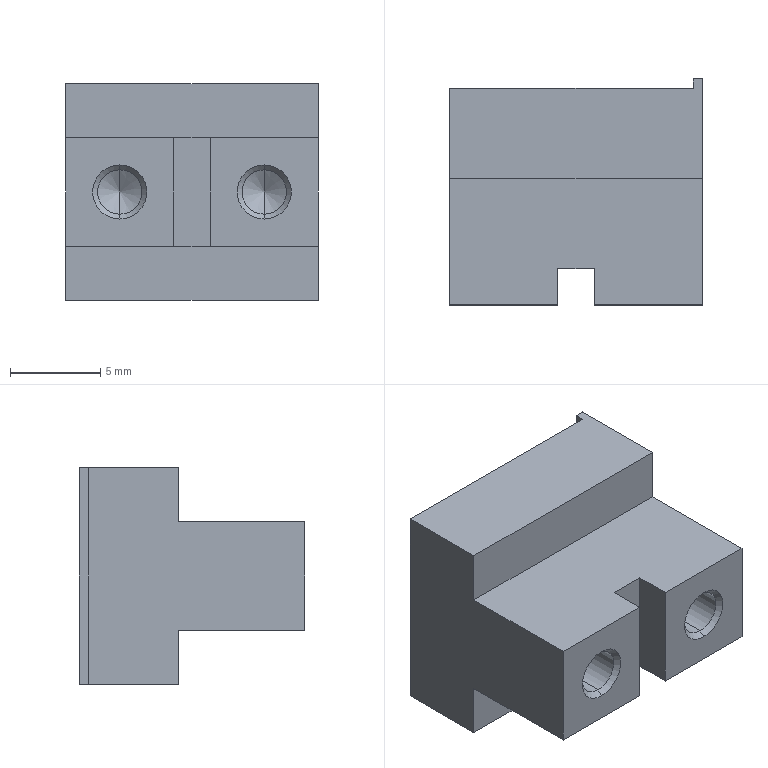Part | SolidWorks | features BaseBody 1 | 1 solid | 28 faces | box 14 x 12.5 x 12 mm | volume 1347 mm3 | plane 16 | cone 8 | cylinder 4 | commonest cylinder face diameters 2.459 x4
STEP:
#1=CARTESIAN_POINT('',(-11.,-11.729,1.229));
#2=VERTEX_POINT('',#1);
#3=CARTESIAN_POINT('',(-11.,-11.729,-1.229));
#4=VERTEX_POINT('',#3);
#5=CARTESIAN_POINT('',(-11.,-11.729,0.));
#6=DIRECTION('',(0.,-1.,0.));
#7=DIRECTION('',(0.,0.,-1.));
#8=AXIS2_PLACEMENT_3D('',#5,#6,#7);
#9=CIRCLE('',#8,1.229);
#10=EDGE_CURVE('',#2,#4,#9,.T.);
#11=ORIENTED_EDGE('',*,*,#10,.F.);
#12=CARTESIAN_POINT('',(-11.,-12.,1.5));
#13=VERTEX_POINT('',#12);
#14=CARTESIAN_POINT('',(-11.,-11.729,1.229));
#15=DIRECTION('',(0.,-0.7071,0.7071));
#16=VECTOR('',#15,1000.);
#17=LINE('',#14,#16);
#18=EDGE_CURVE('',#2,#13,#17,.T.);
#19=ORIENTED_EDGE('',*,*,#18,.T.);
#20=CARTESIAN_POINT('',(-11.,-12.,-1.5));
#21=VERTEX_POINT('',#20);
#22=CARTESIAN_POINT('',(-11.,-12.,0.));
#23=DIRECTION('',(0.,-1.,0.));
#24=DIRECTION('',(0.,0.,-1.));
#25=AXIS2_PLACEMENT_3D('',#22,#23,#24);
#26=CIRCLE('',#25,1.5);
#27=EDGE_CURVE('',#13,#21,#26,.T.);
#28=ORIENTED_EDGE('',*,*,#27,.T.);
#29=CARTESIAN_POINT('',(-11.,-11.729,-1.229));
#30=DIRECTION('',(0.,-0.7071,-0.7071));
#31=VECTOR('',#30,1000.);
#32=LINE('',#29,#31);
#33=EDGE_CURVE('',#4,#21,#32,.T.);
#34=ORIENTED_EDGE('',*,*,#33,.F.);
#35=EDGE_LOOP('',(#11,#19,#28,#34));
#36=FACE_OUTER_BOUND('',#35,.T.);
#37=CARTESIAN_POINT('',(-11.,-11.729,0.));
#38=DIRECTION('',(0.,-1.,0.));
#39=DIRECTION('',(0.,0.,-1.));
#40=AXIS2_PLACEMENT_3D('',#37,#38,#39);
#41=CONICAL_SURFACE('',#40,1.229,0.7854);
#42=ADVANCED_FACE('',(#36),#41,.F.);
#43=CARTESIAN_POINT('',(-11.,-6.,1.229));
#44=VERTEX_POINT('',#43);
#45=CARTESIAN_POINT('',(-11.,-6.,-1.229));
#46=VERTEX_POINT('',#45);
#47=CARTESIAN_POINT('',(-11.,-6.,0.));
#48=DIRECTION('',(0.,-1.,0.));
#49=DIRECTION('',(0.,0.,-1.));
#50=AXIS2_PLACEMENT_3D('',#47,#48,#49);
#51=CIRCLE('',#50,1.229);
#52=EDGE_CURVE('',#44,#46,#51,.T.);
#53=ORIENTED_EDGE('',*,*,#52,.F.);
#54=CARTESIAN_POINT('',(-11.,-12.,1.229));
#55=DIRECTION('',(0.,-1.,0.));
#56=VECTOR('',#55,1000.);
#57=LINE('',#54,#56);
#58=EDGE_CURVE('',#44,#2,#57,.T.);
#59=ORIENTED_EDGE('',*,*,#58,.T.);
#60=ORIENTED_EDGE('',*,*,#10,.T.);
#61=CARTESIAN_POINT('',(-11.,-12.,-1.229));
#62=DIRECTION('',(0.,-1.,0.));
#63=VECTOR('',#62,1000.);
#64=LINE('',#61,#63);
#65=EDGE_CURVE('',#46,#4,#64,.T.);
#66=ORIENTED_EDGE('',*,*,#65,.F.);
#67=EDGE_LOOP('',(#53,#59,#60,#66));
#68=FACE_OUTER_BOUND('',#67,.T.);
#69=CARTESIAN_POINT('',(-11.,-12.,0.));
#70=DIRECTION('',(0.,-1.,0.));
#71=DIRECTION('',(0.,0.,-1.));
#72=AXIS2_PLACEMENT_3D('',#69,#70,#71);
#73=CYLINDRICAL_SURFACE('',#72,1.229);
#74=ADVANCED_FACE('',(#68),#73,.F.);
#75=CARTESIAN_POINT('',(-11.,-5.29,0.));
#76=VERTEX_POINT('',#75);
#77=CARTESIAN_POINT('',(-11.,-5.29,0.));
#78=DIRECTION('',(0.,-0.5,-0.866));
#79=VECTOR('',#78,1000.);
#80=LINE('',#77,#79);
#81=EDGE_CURVE('',#76,#46,#80,.T.);
#82=ORIENTED_EDGE('',*,*,#81,.F.);
#83=CARTESIAN_POINT('',(-11.,-5.29,0.));
#84=DIRECTION('',(0.,-0.5,0.866));
#85=VECTOR('',#84,1000.);
#86=LINE('',#83,#85);
#87=EDGE_CURVE('',#76,#44,#86,.T.);
#88=ORIENTED_EDGE('',*,*,#87,.T.);
#89=ORIENTED_EDGE('',*,*,#52,.T.);
#90=EDGE_LOOP('',(#82,#88,#89));
#91=FACE_OUTER_BOUND('',#90,.T.);
#92=CARTESIAN_POINT('',(-11.,-1005.29,0.));
#93=DIRECTION('',(0.,-1.,0.));
#94=DIRECTION('',(0.,0.,-1.));
#95=AXIS2_PLACEMENT_3D('',#92,#93,#94);
#96=CONICAL_SURFACE('',#95,1732.051,1.047);
#97=ADVANCED_FACE('',(#91),#96,.F.);
#98=CARTESIAN_POINT('',(-3.,-11.729,1.229));
#99=VERTEX_POINT('',#98);
#100=CARTESIAN_POINT('',(-3.,-11.729,-1.229));
#101=VERTEX_POINT('',#100);
#102=CARTESIAN_POINT('',(-3.,-11.729,0.));
#103=DIRECTION('',(0.,-1.,0.));
#104=DIRECTION('',(0.,0.,-1.));
#105=AXIS2_PLACEMENT_3D('',#102,#103,#104);
#106=CIRCLE('',#105,1.229);
#107=EDGE_CURVE('',#99,#101,#106,.T.);
#108=ORIENTED_EDGE('',*,*,#107,.F.);
#109=CARTESIAN_POINT('',(-3.,-12.,1.5));
#110=VERTEX_POINT('',#109);
#111=CARTESIAN_POINT('',(-3.,-11.729,1.229));
#112=DIRECTION('',(0.,-0.7071,0.7071));
#113=VECTOR('',#112,1000.);
#114=LINE('',#111,#113);
#115=EDGE_CURVE('',#99,#110,#114,.T.);
#116=ORIENTED_EDGE('',*,*,#115,.T.);
#117=CARTESIAN_POINT('',(-3.,-12.,-1.5));
#118=VERTEX_POINT('',#117);
#119=CARTESIAN_POINT('',(-3.,-12.,0.));
#120=DIRECTION('',(0.,-1.,0.));
#121=DIRECTION('',(0.,0.,-1.));
#122=AXIS2_PLACEMENT_3D('',#119,#120,#121);
#123=CIRCLE('',#122,1.5);
#124=EDGE_CURVE('',#110,#118,#123,.T.);
#125=ORIENTED_EDGE('',*,*,#124,.T.);
#126=CARTESIAN_POINT('',(-3.,-11.729,-1.229));
#127=DIRECTION('',(0.,-0.7071,-0.7071));
#128=VECTOR('',#127,1000.);
#129=LINE('',#126,#128);
#130=EDGE_CURVE('',#101,#118,#129,.T.);
#131=ORIENTED_EDGE('',*,*,#130,.F.);
#132=EDGE_LOOP('',(#108,#116,#125,#131));
#133=FACE_OUTER_BOUND('',#132,.T.);
#134=CARTESIAN_POINT('',(-3.,-11.729,0.));
#135=DIRECTION('',(0.,-1.,0.));
#136=DIRECTION('',(0.,0.,-1.));
#137=AXIS2_PLACEMENT_3D('',#134,#135,#136);
#138=CONICAL_SURFACE('',#137,1.229,0.7854);
#139=ADVANCED_FACE('',(#133),#138,.F.);
#140=CARTESIAN_POINT('',(-3.,-6.,1.229));
#141=VERTEX_POINT('',#140);
#142=CARTESIAN_POINT('',(-3.,-6.,-1.229));
#143=VERTEX_POINT('',#142);
#144=CARTESIAN_POINT('',(-3.,-6.,0.));
#145=DIRECTION('',(0.,-1.,0.));
#146=DIRECTION('',(0.,0.,-1.));
#147=AXIS2_PLACEMENT_3D('',#144,#145,#146);
#148=CIRCLE('',#147,1.229);
#149=EDGE_CURVE('',#141,#143,#148,.T.);
#150=ORIENTED_EDGE('',*,*,#149,.F.);
#151=CARTESIAN_POINT('',(-3.,-12.,1.229));
#152=DIRECTION('',(0.,-1.,0.));
#153=VECTOR('',#152,1000.);
#154=LINE('',#151,#153);
#155=EDGE_CURVE('',#141,#99,#154,.T.);
#156=ORIENTED_EDGE('',*,*,#155,.T.);
#157=ORIENTED_EDGE('',*,*,#107,.T.);
#158=CARTESIAN_POINT('',(-3.,-12.,-1.229));
#159=DIRECTION('',(0.,-1.,0.));
#160=VECTOR('',#159,1000.);
#161=LINE('',#158,#160);
#162=EDGE_CURVE('',#143,#101,#161,.T.);
#163=ORIENTED_EDGE('',*,*,#162,.F.);
#164=EDGE_LOOP('',(#150,#156,#157,#163));
#165=FACE_OUTER_BOUND('',#164,.T.);
#166=CARTESIAN_POINT('',(-3.,-12.,0.));
#167=DIRECTION('',(0.,-1.,0.));
#168=DIRECTION('',(0.,0.,-1.));
#169=AXIS2_PLACEMENT_3D('',#166,#167,#168);
#170=CYLINDRICAL_SURFACE('',#169,1.229);
#171=ADVANCED_FACE('',(#165),#170,.F.);
#172=CARTESIAN_POINT('',(-3.,-5.29,0.));
#173=VERTEX_POINT('',#172);
#174=CARTESIAN_POINT('',(-3.,-5.29,0.));
#175=DIRECTION('',(0.,-0.5,-0.866));
#176=VECTOR('',#175,1000.);
#177=LINE('',#174,#176);
#178=EDGE_CURVE('',#173,#143,#177,.T.);
#179=ORIENTED_EDGE('',*,*,#178,.F.);
#180=CARTESIAN_POINT('',(-3.,-5.29,0.));
#181=DIRECTION('',(0.,-0.5,0.866));
#182=VECTOR('',#181,1000.);
#183=LINE('',#180,#182);
#184=EDGE_CURVE('',#173,#141,#183,.T.);
#185=ORIENTED_EDGE('',*,*,#184,.T.);
#186=ORIENTED_EDGE('',*,*,#149,.T.);
#187=EDGE_LOOP('',(#179,#185,#186));
#188=FACE_OUTER_BOUND('',#187,.T.);
#189=CARTESIAN_POINT('',(-3.,-1005.29,0.));
#190=DIRECTION('',(0.,-1.,0.));
#191=DIRECTION('',(0.,0.,-1.));
#192=AXIS2_PLACEMENT_3D('',#189,#190,#191);
#193=CONICAL_SURFACE('',#192,1732.051,1.047);
#194=ADVANCED_FACE('',(#188),#193,.F.);
#195=CARTESIAN_POINT('',(-3.,-12.,0.));
#196=DIRECTION('',(0.,-1.,0.));
#197=DIRECTION('',(0.,0.,-1.));
#198=AXIS2_PLACEMENT_3D('',#195,#196,#197);
#199=CIRCLE('',#198,1.5);
#200=EDGE_CURVE('',#118,#110,#199,.T.);
#201=ORIENTED_EDGE('',*,*,#200,.F.);
#202=ORIENTED_EDGE('',*,*,#124,.F.);
#203=EDGE_LOOP('',(#201,#202));
#204=FACE_BOUND('',#203,.T.);
#205=CARTESIAN_POINT('',(-6.,-12.,-3.));
#206=VERTEX_POINT('',#205);
#207=CARTESIAN_POINT('',(-6.,-12.,3.));
#208=VERTEX_POINT('',#207);
#209=CARTESIAN_POINT('',(-6.,-12.,-3.));
#210=DIRECTION('',(0.,0.,1.));
#211=VECTOR('',#210,1000.);
#212=LINE('',#209,#211);
#213=EDGE_CURVE('',#206,#208,#212,.T.);
#214=ORIENTED_EDGE('',*,*,#213,.F.);
#215=CARTESIAN_POINT('',(0.,-12.,-3.));
#216=VERTEX_POINT('',#215);
#217=CARTESIAN_POINT('',(-6.,-12.,-3.));
#218=DIRECTION('',(1.,0.,0.));
#219=VECTOR('',#218,1000.);
#220=LINE('',#217,#219);
#221=EDGE_CURVE('',#206,#216,#220,.T.);
#222=ORIENTED_EDGE('',*,*,#221,.T.);
#223=CARTESIAN_POINT('',(0.,-12.,3.));
#224=VERTEX_POINT('',#223);
#225=CARTESIAN_POINT('',(0.,-12.,3.));
#226=DIRECTION('',(0.,0.,-1.));
#227=VECTOR('',#226,1000.);
#228=LINE('',#225,#227);
#229=EDGE_CURVE('',#224,#216,#228,.T.);
#230=ORIENTED_EDGE('',*,*,#229,.F.);
#231=CARTESIAN_POINT('',(-6.,-12.,3.));
#232=DIRECTION('',(1.,0.,0.));
#233=VECTOR('',#232,1000.);
#234=LINE('',#231,#233);
#235=EDGE_CURVE('',#208,#224,#234,.T.);
#236=ORIENTED_EDGE('',*,*,#235,.F.);
#237=EDGE_LOOP('',(#214,#222,#230,#236));
#238=FACE_OUTER_BOUND('',#237,.T.);
#239=CARTESIAN_POINT('',(-14.,-12.,3.));
#240=DIRECTION('',(0.,-1.,0.));
#241=DIRECTION('',(0.,0.,-1.));
#242=AXIS2_PLACEMENT_3D('',#239,#240,#241);
#243=PLANE('',#242);
#244=ADVANCED_FACE('',(#204,#238),#243,.T.);
#245=CARTESIAN_POINT('',(-14.,0.,6.));
#246=VERTEX_POINT('',#245);
#247=CARTESIAN_POINT('',(-0.5,0.,6.));
#248=VERTEX_POINT('',#247);
#249=CARTESIAN_POINT('',(-14.,0.,6.));
#250=DIRECTION('',(1.,0.,0.));
#251=VECTOR('',#250,1000.);
#252=LINE('',#249,#251);
#253=EDGE_CURVE('',#246,#248,#252,.T.);
#254=ORIENTED_EDGE('',*,*,#253,.T.);
#255=CARTESIAN_POINT('',(-0.5,0.,-6.));
#256=VERTEX_POINT('',#255);
#257=CARTESIAN_POINT('',(-0.5,0.,6.));
#258=DIRECTION('',(0.,0.,-1.));
#259=VECTOR('',#258,1000.);
#260=LINE('',#257,#259);
#261=EDGE_CURVE('',#248,#256,#260,.T.);
#262=ORIENTED_EDGE('',*,*,#261,.T.);
#263=CARTESIAN_POINT('',(-14.,0.,-6.));
#264=VERTEX_POINT('',#263);
#265=CARTESIAN_POINT('',(-14.,0.,-6.));
#266=DIRECTION('',(1.,0.,0.));
#267=VECTOR('',#266,1000.);
#268=LINE('',#265,#267);
#269=EDGE_CURVE('',#264,#256,#268,.T.);
#270=ORIENTED_EDGE('',*,*,#269,.F.);
#271=CARTESIAN_POINT('',(-14.,0.,-6.));
#272=DIRECTION('',(0.,0.,1.));
#273=VECTOR('',#272,1000.);
#274=LINE('',#271,#273);
#275=EDGE_CURVE('',#264,#246,#274,.T.);
#276=ORIENTED_EDGE('',*,*,#275,.T.);
#277=EDGE_LOOP('',(#254,#262,#270,#276));
#278=FACE_OUTER_BOUND('',#277,.T.);
#279=CARTESIAN_POINT('',(-14.,0.,-6.));
#280=DIRECTION('',(0.,1.,0.));
#281=DIRECTION('',(0.,0.,1.));
#282=AXIS2_PLACEMENT_3D('',#279,#280,#281);
#283=PLANE('',#282);
#284=ADVANCED_FACE('',(#278),#283,.T.);
#285=CARTESIAN_POINT('',(0.,0.5,6.));
#286=VERTEX_POINT('',#285);
#287=CARTESIAN_POINT('',(0.,-5.,6.));
#288=VERTEX_POINT('',#287);
#289=CARTESIAN_POINT('',(0.,0.5,6.));
#290=DIRECTION('',(0.,-1.,0.));
#291=VECTOR('',#290,1000.);
#292=LINE('',#289,#291);
#293=EDGE_CURVE('',#286,#288,#292,.T.);
#294=ORIENTED_EDGE('',*,*,#293,.F.);
#295=CARTESIAN_POINT('',(-0.5,0.5,6.));
#296=VERTEX_POINT('',#295);
#297=CARTESIAN_POINT('',(-0.5,0.5,6.));
#298=DIRECTION('',(1.,0.,0.));
#299=VECTOR('',#298,1000.);
#300=LINE('',#297,#299);
#301=EDGE_CURVE('',#296,#286,#300,.T.);
#302=ORIENTED_EDGE('',*,*,#301,.F.);
#303=CARTESIAN_POINT('',(-0.5,0.5,6.));
#304=DIRECTION('',(0.,-1.,0.));
#305=VECTOR('',#304,1000.);
#306=LINE('',#303,#305);
#307=EDGE_CURVE('',#296,#248,#306,.T.);
#308=ORIENTED_EDGE('',*,*,#307,.T.);
#309=ORIENTED_EDGE('',*,*,#253,.F.);
#310=CARTESIAN_POINT('',(-14.,-5.,6.));
#311=VERTEX_POINT('',#310);
#312=CARTESIAN_POINT('',(-14.,0.,6.));
#313=DIRECTION('',(0.,-1.,0.));
#314=VECTOR('',#313,1000.);
#315=LINE('',#312,#314);
#316=EDGE_CURVE('',#246,#311,#315,.T.);
#317=ORIENTED_EDGE('',*,*,#316,.T.);
#318=CARTESIAN_POINT('',(-14.,-5.,6.));
#319=DIRECTION('',(1.,0.,0.));
#320=VECTOR('',#319,1000.);
#321=LINE('',#318,#320);
#322=EDGE_CURVE('',#311,#288,#321,.T.);
#323=ORIENTED_EDGE('',*,*,#322,.T.);
#324=EDGE_LOOP('',(#294,#302,#308,#309,#317,#323));
#325=FACE_OUTER_BOUND('',#324,.T.);
#326=CARTESIAN_POINT('',(-14.,0.,6.));
#327=DIRECTION('',(0.,0.,1.));
#328=DIRECTION('',(1.,0.,0.));
#329=AXIS2_PLACEMENT_3D('',#326,#327,#328);
#330=PLANE('',#329);
#331=ADVANCED_FACE('',(#325),#330,.T.);
#332=CARTESIAN_POINT('',(0.,-5.,3.));
#333=VERTEX_POINT('',#332);
#334=CARTESIAN_POINT('',(0.,-5.,6.));
#335=DIRECTION('',(0.,0.,-1.));
#336=VECTOR('',#335,1000.);
#337=LINE('',#334,#336);
#338=EDGE_CURVE('',#288,#333,#337,.T.);
#339=ORIENTED_EDGE('',*,*,#338,.F.);
#340=ORIENTED_EDGE('',*,*,#322,.F.);
#341=CARTESIAN_POINT('',(-14.,-5.,3.));
#342=VERTEX_POINT('',#341);
#343=CARTESIAN_POINT('',(-14.,-5.,6.));
#344=DIRECTION('',(0.,0.,-1.));
#345=VECTOR('',#344,1000.);
#346=LINE('',#343,#345);
#347=EDGE_CURVE('',#311,#342,#346,.T.);
#348=ORIENTED_EDGE('',*,*,#347,.T.);
#349=CARTESIAN_POINT('',(-14.,-5.,3.));
#350=DIRECTION('',(1.,0.,0.));
#351=VECTOR('',#350,1000.);
#352=LINE('',#349,#351);
#353=EDGE_CURVE('',#342,#333,#352,.T.);
#354=ORIENTED_EDGE('',*,*,#353,.T.);
#355=EDGE_LOOP('',(#339,#340,#348,#354));
#356=FACE_OUTER_BOUND('',#355,.T.);
#357=CARTESIAN_POINT('',(-14.,-5.,6.));
#358=DIRECTION('',(0.,-1.,0.));
#359=DIRECTION('',(0.,0.,-1.));
#360=AXIS2_PLACEMENT_3D('',#357,#358,#359);
#361=PLANE('',#360);
#362=ADVANCED_FACE('',(#356),#361,.T.);
#363=CARTESIAN_POINT('',(-6.,-10.,3.));
#364=VERTEX_POINT('',#363);
#365=CARTESIAN_POINT('',(-6.,-10.,3.));
#366=DIRECTION('',(0.,-1.,0.));
#367=VECTOR('',#366,1000.);
#368=LINE('',#365,#367);
#369=EDGE_CURVE('',#364,#208,#368,.T.);
#370=ORIENTED_EDGE('',*,*,#369,.T.);
#371=ORIENTED_EDGE('',*,*,#235,.T.);
#372=CARTESIAN_POINT('',(0.,-5.,3.));
#373=DIRECTION('',(0.,-1.,0.));
#374=VECTOR('',#373,1000.);
#375=LINE('',#372,#374);
#376=EDGE_CURVE('',#333,#224,#375,.T.);
#377=ORIENTED_EDGE('',*,*,#376,.F.);
#378=ORIENTED_EDGE('',*,*,#353,.F.);
#379=CARTESIAN_POINT('',(-14.,-12.,3.));
#380=VERTEX_POINT('',#379);
#381=CARTESIAN_POINT('',(-14.,-5.,3.));
#382=DIRECTION('',(0.,-1.,0.));
#383=VECTOR('',#382,1000.);
#384=LINE('',#381,#383);
#385=EDGE_CURVE('',#342,#380,#384,.T.);
#386=ORIENTED_EDGE('',*,*,#385,.T.);
#387=CARTESIAN_POINT('',(-8.,-12.,3.));
#388=VERTEX_POINT('',#387);
#389=CARTESIAN_POINT('',(-14.,-12.,3.));
#390=DIRECTION('',(1.,0.,0.));
#391=VECTOR('',#390,1000.);
#392=LINE('',#389,#391);
#393=EDGE_CURVE('',#380,#388,#392,.T.);
#394=ORIENTED_EDGE('',*,*,#393,.T.);
#395=CARTESIAN_POINT('',(-8.,-10.,3.));
#396=VERTEX_POINT('',#395);
#397=CARTESIAN_POINT('',(-8.,-10.,3.));
#398=DIRECTION('',(0.,-1.,0.));
#399=VECTOR('',#398,1000.);
#400=LINE('',#397,#399);
#401=EDGE_CURVE('',#396,#388,#400,.T.);
#402=ORIENTED_EDGE('',*,*,#401,.F.);
#403=CARTESIAN_POINT('',(-6.,-10.,3.));
#404=DIRECTION('',(-1.,0.,0.));
#405=VECTOR('',#404,1000.);
#406=LINE('',#403,#405);
#407=EDGE_CURVE('',#364,#396,#406,.T.);
#408=ORIENTED_EDGE('',*,*,#407,.F.);
#409=EDGE_LOOP('',(#370,#371,#377,#378,#386,#394,#402,#408));
#410=FACE_OUTER_BOUND('',#409,.T.);
#411=CARTESIAN_POINT('',(-14.,-5.,3.));
#412=DIRECTION('',(0.,0.,1.));
#413=DIRECTION('',(1.,0.,0.));
#414=AXIS2_PLACEMENT_3D('',#411,#412,#413);
#415=PLANE('',#414);
#416=ADVANCED_FACE('',(#410),#415,.T.);
#417=CARTESIAN_POINT('',(-11.,-12.,0.));
#418=DIRECTION('',(0.,-1.,0.));
#419=DIRECTION('',(0.,0.,-1.));
#420=AXIS2_PLACEMENT_3D('',#417,#418,#419);
#421=CIRCLE('',#420,1.5);
#422=EDGE_CURVE('',#21,#13,#421,.T.);
#423=ORIENTED_EDGE('',*,*,#422,.F.);
#424=ORIENTED_EDGE('',*,*,#27,.F.);
#425=EDGE_LOOP('',(#423,#424));
#426=FACE_BOUND('',#425,.T.);
#427=CARTESIAN_POINT('',(-8.,-12.,-3.));
#428=VERTEX_POINT('',#427);
#429=CARTESIAN_POINT('',(-8.,-12.,3.));
#430=DIRECTION('',(0.,0.,-1.));
#431=VECTOR('',#430,1000.);
#432=LINE('',#429,#431);
#433=EDGE_CURVE('',#388,#428,#432,.T.);
#434=ORIENTED_EDGE('',*,*,#433,.F.);
#435=ORIENTED_EDGE('',*,*,#393,.F.);
#436=CARTESIAN_POINT('',(-14.,-12.,-3.));
#437=VERTEX_POINT('',#436);
#438=CARTESIAN_POINT('',(-14.,-12.,3.));
#439=DIRECTION('',(0.,0.,-1.));
#440=VECTOR('',#439,1000.);
#441=LINE('',#438,#440);
#442=EDGE_CURVE('',#380,#437,#441,.T.);
#443=ORIENTED_EDGE('',*,*,#442,.T.);
#444=CARTESIAN_POINT('',(-14.,-12.,-3.));
#445=DIRECTION('',(1.,0.,0.));
#446=VECTOR('',#445,1000.);
#447=LINE('',#444,#446);
#448=EDGE_CURVE('',#437,#428,#447,.T.);
#449=ORIENTED_EDGE('',*,*,#448,.T.);
#450=EDGE_LOOP('',(#434,#435,#443,#449));
#451=FACE_OUTER_BOUND('',#450,.T.);
#452=CARTESIAN_POINT('',(-14.,-12.,3.));
#453=DIRECTION('',(0.,-1.,0.));
#454=DIRECTION('',(0.,0.,-1.));
#455=AXIS2_PLACEMENT_3D('',#452,#453,#454);
#456=PLANE('',#455);
#457=ADVANCED_FACE('',(#426,#451),#456,.T.);
#458=CARTESIAN_POINT('',(-6.,-10.,-3.));
#459=VERTEX_POINT('',#458);
#460=CARTESIAN_POINT('',(-6.,-10.,-3.));
#461=DIRECTION('',(0.,-1.,0.));
#462=VECTOR('',#461,1000.);
#463=LINE('',#460,#462);
#464=EDGE_CURVE('',#459,#206,#463,.T.);
#465=ORIENTED_EDGE('',*,*,#464,.F.);
#466=CARTESIAN_POINT('',(-8.,-10.,-3.));
#467=VERTEX_POINT('',#466);
#468=CARTESIAN_POINT('',(-8.,-10.,-3.));
#469=DIRECTION('',(1.,0.,0.));
#470=VECTOR('',#469,1000.);
#471=LINE('',#468,#470);
#472=EDGE_CURVE('',#467,#459,#471,.T.);
#473=ORIENTED_EDGE('',*,*,#472,.F.);
#474=CARTESIAN_POINT('',(-8.,-10.,-3.));
#475=DIRECTION('',(0.,-1.,0.));
#476=VECTOR('',#475,1000.);
#477=LINE('',#474,#476);
#478=EDGE_CURVE('',#467,#428,#477,.T.);
#479=ORIENTED_EDGE('',*,*,#478,.T.);
#480=ORIENTED_EDGE('',*,*,#448,.F.);
#481=CARTESIAN_POINT('',(-14.,-5.,-3.));
#482=VERTEX_POINT('',#481);
#483=CARTESIAN_POINT('',(-14.,-12.,-3.));
#484=DIRECTION('',(0.,1.,0.));
#485=VECTOR('',#484,1000.);
#486=LINE('',#483,#485);
#487=EDGE_CURVE('',#437,#482,#486,.T.);
#488=ORIENTED_EDGE('',*,*,#487,.T.);
#489=CARTESIAN_POINT('',(0.,-5.,-3.));
#490=VERTEX_POINT('',#489);
#491=CARTESIAN_POINT('',(-14.,-5.,-3.));
#492=DIRECTION('',(1.,0.,0.));
#493=VECTOR('',#492,1000.);
#494=LINE('',#491,#493);
#495=EDGE_CURVE('',#482,#490,#494,.T.);
#496=ORIENTED_EDGE('',*,*,#495,.T.);
#497=CARTESIAN_POINT('',(0.,-12.,-3.));
#498=DIRECTION('',(0.,1.,0.));
#499=VECTOR('',#498,1000.);
#500=LINE('',#497,#499);
#501=EDGE_CURVE('',#216,#490,#500,.T.);
#502=ORIENTED_EDGE('',*,*,#501,.F.);
#503=ORIENTED_EDGE('',*,*,#221,.F.);
#504=EDGE_LOOP('',(#465,#473,#479,#480,#488,#496,#502,#503));
#505=FACE_OUTER_BOUND('',#504,.T.);
#506=CARTESIAN_POINT('',(-14.,-12.,-3.));
#507=DIRECTION('',(0.,0.,-1.));
#508=DIRECTION('',(-1.,0.,0.));
#509=AXIS2_PLACEMENT_3D('',#506,#507,#508);
#510=PLANE('',#509);
#511=ADVANCED_FACE('',(#505),#510,.T.);
#512=CARTESIAN_POINT('',(0.,-5.,-6.));
#513=VERTEX_POINT('',#512);
#514=CARTESIAN_POINT('',(0.,-5.,-3.));
#515=DIRECTION('',(0.,0.,-1.));
#516=VECTOR('',#515,1000.);
#517=LINE('',#514,#516);
#518=EDGE_CURVE('',#490,#513,#517,.T.);
#519=ORIENTED_EDGE('',*,*,#518,.F.);
#520=ORIENTED_EDGE('',*,*,#495,.F.);
#521=CARTESIAN_POINT('',(-14.,-5.,-6.));
#522=VERTEX_POINT('',#521);
#523=CARTESIAN_POINT('',(-14.,-5.,-3.));
#524=DIRECTION('',(0.,0.,-1.));
#525=VECTOR('',#524,1000.);
#526=LINE('',#523,#525);
#527=EDGE_CURVE('',#482,#522,#526,.T.);
#528=ORIENTED_EDGE('',*,*,#527,.T.);
#529=CARTESIAN_POINT('',(-14.,-5.,-6.));
#530=DIRECTION('',(1.,0.,0.));
#531=VECTOR('',#530,1000.);
#532=LINE('',#529,#531);
#533=EDGE_CURVE('',#522,#513,#532,.T.);
#534=ORIENTED_EDGE('',*,*,#533,.T.);
#535=EDGE_LOOP('',(#519,#520,#528,#534));
#536=FACE_OUTER_BOUND('',#535,.T.);
#537=CARTESIAN_POINT('',(-14.,-5.,-3.));
#538=DIRECTION('',(0.,-1.,0.));
#539=DIRECTION('',(0.,0.,-1.));
#540=AXIS2_PLACEMENT_3D('',#537,#538,#539);
#541=PLANE('',#540);
#542=ADVANCED_FACE('',(#536),#541,.T.);
#543=CARTESIAN_POINT('',(0.,0.5,-6.));
#544=VERTEX_POINT('',#543);
#545=CARTESIAN_POINT('',(0.,-5.,-6.));
#546=DIRECTION('',(0.,1.,0.));
#547=VECTOR('',#546,1000.);
#548=LINE('',#545,#547);
#549=EDGE_CURVE('',#513,#544,#548,.T.);
#550=ORIENTED_EDGE('',*,*,#549,.F.);
#551=ORIENTED_EDGE('',*,*,#533,.F.);
#552=CARTESIAN_POINT('',(-14.,-5.,-6.));
#553=DIRECTION('',(0.,1.,0.));
#554=VECTOR('',#553,1000.);
#555=LINE('',#552,#554);
#556=EDGE_CURVE('',#522,#264,#555,.T.);
#557=ORIENTED_EDGE('',*,*,#556,.T.);
#558=ORIENTED_EDGE('',*,*,#269,.T.);
#559=CARTESIAN_POINT('',(-0.5,0.5,-6.));
#560=VERTEX_POINT('',#559);
#561=CARTESIAN_POINT('',(-0.5,0.,-6.));
#562=DIRECTION('',(0.,1.,0.));
#563=VECTOR('',#562,1000.);
#564=LINE('',#561,#563);
#565=EDGE_CURVE('',#256,#560,#564,.T.);
#566=ORIENTED_EDGE('',*,*,#565,.T.);
#567=CARTESIAN_POINT('',(-0.5,0.5,-6.));
#568=DIRECTION('',(1.,0.,0.));
#569=VECTOR('',#568,1000.);
#570=LINE('',#567,#569);
#571=EDGE_CURVE('',#560,#544,#570,.T.);
#572=ORIENTED_EDGE('',*,*,#571,.T.);
#573=EDGE_LOOP('',(#550,#551,#557,#558,#566,#572));
#574=FACE_OUTER_BOUND('',#573,.T.);
#575=CARTESIAN_POINT('',(-14.,-5.,-6.));
#576=DIRECTION('',(0.,0.,-1.));
#577=DIRECTION('',(-1.,0.,0.));
#578=AXIS2_PLACEMENT_3D('',#575,#576,#577);
#579=PLANE('',#578);
#580=ADVANCED_FACE('',(#574),#579,.T.);
#581=ORIENTED_EDGE('',*,*,#316,.F.);
#582=ORIENTED_EDGE('',*,*,#275,.F.);
#583=ORIENTED_EDGE('',*,*,#556,.F.);
#584=ORIENTED_EDGE('',*,*,#527,.F.);
#585=ORIENTED_EDGE('',*,*,#487,.F.);
#586=ORIENTED_EDGE('',*,*,#442,.F.);
#587=ORIENTED_EDGE('',*,*,#385,.F.);
#588=ORIENTED_EDGE('',*,*,#347,.F.);
#589=EDGE_LOOP('',(#581,#582,#583,#584,#585,#586,#587,#588));
#590=FACE_OUTER_BOUND('',#589,.T.);
#591=CARTESIAN_POINT('',(-14.,0.,0.));
#592=DIRECTION('',(1.,0.,0.));
#593=DIRECTION('',(0.,0.,-1.));
#594=AXIS2_PLACEMENT_3D('',#591,#592,#593);
#595=PLANE('',#594);
#596=ADVANCED_FACE('',(#590),#595,.F.);
#597=ORIENTED_EDGE('',*,*,#293,.T.);
#598=ORIENTED_EDGE('',*,*,#338,.T.);
#599=ORIENTED_EDGE('',*,*,#376,.T.);
#600=ORIENTED_EDGE('',*,*,#229,.T.);
#601=ORIENTED_EDGE('',*,*,#501,.T.);
#602=ORIENTED_EDGE('',*,*,#518,.T.);
#603=ORIENTED_EDGE('',*,*,#549,.T.);
#604=CARTESIAN_POINT('',(0.,0.5,-6.));
#605=DIRECTION('',(0.,0.,1.));
#606=VECTOR('',#605,1000.);
#607=LINE('',#604,#606);
#608=EDGE_CURVE('',#544,#286,#607,.T.);
#609=ORIENTED_EDGE('',*,*,#608,.T.);
#610=EDGE_LOOP('',(#597,#598,#599,#600,#601,#602,#603,#609));
#611=FACE_OUTER_BOUND('',#610,.T.);
#612=CARTESIAN_POINT('',(0.,0.,0.));
#613=DIRECTION('',(1.,0.,0.));
#614=DIRECTION('',(0.,0.,-1.));
#615=AXIS2_PLACEMENT_3D('',#612,#613,#614);
#616=PLANE('',#615);
#617=ADVANCED_FACE('',(#611),#616,.T.);
#618=ORIENTED_EDGE('',*,*,#608,.F.);
#619=ORIENTED_EDGE('',*,*,#571,.F.);
#620=CARTESIAN_POINT('',(-0.5,0.5,-6.));
#621=DIRECTION('',(0.,0.,1.));
#622=VECTOR('',#621,1000.);
#623=LINE('',#620,#622);
#624=EDGE_CURVE('',#560,#296,#623,.T.);
#625=ORIENTED_EDGE('',*,*,#624,.T.);
#626=ORIENTED_EDGE('',*,*,#301,.T.);
#627=EDGE_LOOP('',(#618,#619,#625,#626));
#628=FACE_OUTER_BOUND('',#627,.T.);
#629=CARTESIAN_POINT('',(-0.5,0.5,-6.));
#630=DIRECTION('',(0.,1.,0.));
#631=DIRECTION('',(0.,0.,1.));
#632=AXIS2_PLACEMENT_3D('',#629,#630,#631);
#633=PLANE('',#632);
#634=ADVANCED_FACE('',(#628),#633,.T.);
#635=ORIENTED_EDGE('',*,*,#624,.F.);
#636=ORIENTED_EDGE('',*,*,#565,.F.);
#637=ORIENTED_EDGE('',*,*,#261,.F.);
#638=ORIENTED_EDGE('',*,*,#307,.F.);
#639=EDGE_LOOP('',(#635,#636,#637,#638));
#640=FACE_OUTER_BOUND('',#639,.T.);
#641=CARTESIAN_POINT('',(-0.5,0.,0.));
#642=DIRECTION('',(1.,0.,0.));
#643=DIRECTION('',(0.,0.,-1.));
#644=AXIS2_PLACEMENT_3D('',#641,#642,#643);
#645=PLANE('',#644);
#646=ADVANCED_FACE('',(#640),#645,.F.);
#647=ORIENTED_EDGE('',*,*,#213,.T.);
#648=ORIENTED_EDGE('',*,*,#369,.F.);
#649=CARTESIAN_POINT('',(-6.,-10.,-3.));
#650=DIRECTION('',(0.,0.,1.));
#651=VECTOR('',#650,1000.);
#652=LINE('',#649,#651);
#653=EDGE_CURVE('',#459,#364,#652,.T.);
#654=ORIENTED_EDGE('',*,*,#653,.F.);
#655=ORIENTED_EDGE('',*,*,#464,.T.);
#656=EDGE_LOOP('',(#647,#648,#654,#655));
#657=FACE_OUTER_BOUND('',#656,.T.);
#658=CARTESIAN_POINT('',(-6.,-10.,-3.));
#659=DIRECTION('',(1.,0.,0.));
#660=DIRECTION('',(0.,0.,-1.));
#661=AXIS2_PLACEMENT_3D('',#658,#659,#660);
#662=PLANE('',#661);
#663=ADVANCED_FACE('',(#657),#662,.F.);
#664=ORIENTED_EDGE('',*,*,#433,.T.);
#665=ORIENTED_EDGE('',*,*,#478,.F.);
#666=CARTESIAN_POINT('',(-8.,-10.,3.));
#667=DIRECTION('',(0.,0.,-1.));
#668=VECTOR('',#667,1000.);
#669=LINE('',#666,#668);
#670=EDGE_CURVE('',#396,#467,#669,.T.);
#671=ORIENTED_EDGE('',*,*,#670,.F.);
#672=ORIENTED_EDGE('',*,*,#401,.T.);
#673=EDGE_LOOP('',(#664,#665,#671,#672));
#674=FACE_OUTER_BOUND('',#673,.T.);
#675=CARTESIAN_POINT('',(-8.,-10.,3.));
#676=DIRECTION('',(-1.,0.,0.));
#677=DIRECTION('',(0.,0.,1.));
#678=AXIS2_PLACEMENT_3D('',#675,#676,#677);
#679=PLANE('',#678);
#680=ADVANCED_FACE('',(#674),#679,.F.);
#681=ORIENTED_EDGE('',*,*,#472,.T.);
#682=ORIENTED_EDGE('',*,*,#653,.T.);
#683=ORIENTED_EDGE('',*,*,#407,.T.);
#684=ORIENTED_EDGE('',*,*,#670,.T.);
#685=EDGE_LOOP('',(#681,#682,#683,#684));
#686=FACE_OUTER_BOUND('',#685,.T.);
#687=CARTESIAN_POINT('',(0.,-10.,0.));
#688=DIRECTION('',(0.,-1.,0.));
#689=DIRECTION('',(0.,0.,-1.));
#690=AXIS2_PLACEMENT_3D('',#687,#688,#689);
#691=PLANE('',#690);
#692=ADVANCED_FACE('',(#686),#691,.T.);
#693=ORIENTED_EDGE('',*,*,#184,.F.);
#694=ORIENTED_EDGE('',*,*,#178,.T.);
#695=CARTESIAN_POINT('',(-3.,-6.,0.));
#696=DIRECTION('',(0.,-1.,0.));
#697=DIRECTION('',(0.,0.,-1.));
#698=AXIS2_PLACEMENT_3D('',#695,#696,#697);
#699=CIRCLE('',#698,1.229);
#700=EDGE_CURVE('',#143,#141,#699,.T.);
#701=ORIENTED_EDGE('',*,*,#700,.T.);
#702=EDGE_LOOP('',(#693,#694,#701));
#703=FACE_OUTER_BOUND('',#702,.T.);
#704=CARTESIAN_POINT('',(-3.,-1005.29,0.));
#705=DIRECTION('',(0.,-1.,0.));
#706=DIRECTION('',(0.,0.,-1.));
#707=AXIS2_PLACEMENT_3D('',#704,#705,#706);
#708=CONICAL_SURFACE('',#707,1732.051,1.047);
#709=ADVANCED_FACE('',(#703),#708,.F.);
#710=ORIENTED_EDGE('',*,*,#155,.F.);
#711=ORIENTED_EDGE('',*,*,#700,.F.);
#712=ORIENTED_EDGE('',*,*,#162,.T.);
#713=CARTESIAN_POINT('',(-3.,-11.729,0.));
#714=DIRECTION('',(0.,-1.,0.));
#715=DIRECTION('',(0.,0.,-1.));
#716=AXIS2_PLACEMENT_3D('',#713,#714,#715);
#717=CIRCLE('',#716,1.229);
#718=EDGE_CURVE('',#101,#99,#717,.T.);
#719=ORIENTED_EDGE('',*,*,#718,.T.);
#720=EDGE_LOOP('',(#710,#711,#712,#719));
#721=FACE_OUTER_BOUND('',#720,.T.);
#722=CARTESIAN_POINT('',(-3.,-12.,0.));
#723=DIRECTION('',(0.,-1.,0.));
#724=DIRECTION('',(0.,0.,-1.));
#725=AXIS2_PLACEMENT_3D('',#722,#723,#724);
#726=CYLINDRICAL_SURFACE('',#725,1.229);
#727=ADVANCED_FACE('',(#721),#726,.F.);
#728=ORIENTED_EDGE('',*,*,#115,.F.);
#729=ORIENTED_EDGE('',*,*,#718,.F.);
#730=ORIENTED_EDGE('',*,*,#130,.T.);
#731=ORIENTED_EDGE('',*,*,#200,.T.);
#732=EDGE_LOOP('',(#728,#729,#730,#731));
#733=FACE_OUTER_BOUND('',#732,.T.);
#734=CARTESIAN_POINT('',(-3.,-11.729,0.));
#735=DIRECTION('',(0.,-1.,0.));
#736=DIRECTION('',(0.,0.,-1.));
#737=AXIS2_PLACEMENT_3D('',#734,#735,#736);
#738=CONICAL_SURFACE('',#737,1.229,0.7854);
#739=ADVANCED_FACE('',(#733),#738,.F.);
#740=ORIENTED_EDGE('',*,*,#87,.F.);
#741=ORIENTED_EDGE('',*,*,#81,.T.);
#742=CARTESIAN_POINT('',(-11.,-6.,0.));
#743=DIRECTION('',(0.,-1.,0.));
#744=DIRECTION('',(0.,0.,-1.));
#745=AXIS2_PLACEMENT_3D('',#742,#743,#744);
#746=CIRCLE('',#745,1.229);
#747=EDGE_CURVE('',#46,#44,#746,.T.);
#748=ORIENTED_EDGE('',*,*,#747,.T.);
#749=EDGE_LOOP('',(#740,#741,#748));
#750=FACE_OUTER_BOUND('',#749,.T.);
#751=CARTESIAN_POINT('',(-11.,-1005.29,0.));
#752=DIRECTION('',(0.,-1.,0.));
#753=DIRECTION('',(0.,0.,-1.));
#754=AXIS2_PLACEMENT_3D('',#751,#752,#753);
#755=CONICAL_SURFACE('',#754,1732.051,1.047);
#756=ADVANCED_FACE('',(#750),#755,.F.);
#757=ORIENTED_EDGE('',*,*,#58,.F.);
#758=ORIENTED_EDGE('',*,*,#747,.F.);
#759=ORIENTED_EDGE('',*,*,#65,.T.);
#760=CARTESIAN_POINT('',(-11.,-11.729,0.));
#761=DIRECTION('',(0.,-1.,0.));
#762=DIRECTION('',(0.,0.,-1.));
#763=AXIS2_PLACEMENT_3D('',#760,#761,#762);
#764=CIRCLE('',#763,1.229);
#765=EDGE_CURVE('',#4,#2,#764,.T.);
#766=ORIENTED_EDGE('',*,*,#765,.T.);
#767=EDGE_LOOP('',(#757,#758,#759,#766));
#768=FACE_OUTER_BOUND('',#767,.T.);
#769=CARTESIAN_POINT('',(-11.,-12.,0.));
#770=DIRECTION('',(0.,-1.,0.));
#771=DIRECTION('',(0.,0.,-1.));
#772=AXIS2_PLACEMENT_3D('',#769,#770,#771);
#773=CYLINDRICAL_SURFACE('',#772,1.229);
#774=ADVANCED_FACE('',(#768),#773,.F.);
#775=ORIENTED_EDGE('',*,*,#18,.F.);
#776=ORIENTED_EDGE('',*,*,#765,.F.);
#777=ORIENTED_EDGE('',*,*,#33,.T.);
#778=ORIENTED_EDGE('',*,*,#422,.T.);
#779=EDGE_LOOP('',(#775,#776,#777,#778));
#780=FACE_OUTER_BOUND('',#779,.T.);
#781=CARTESIAN_POINT('',(-11.,-11.729,0.));
#782=DIRECTION('',(0.,-1.,0.));
#783=DIRECTION('',(0.,0.,-1.));
#784=AXIS2_PLACEMENT_3D('',#781,#782,#783);
#785=CONICAL_SURFACE('',#784,1.229,0.7854);
#786=ADVANCED_FACE('',(#780),#785,.F.);
#787=CLOSED_SHELL('',(#42,#74,#97,#139,#171,#194,#244,#284,#331,#362,#416,#457,#511,#542,#580,#596,#617,#634,#646,#663,#680,#692,#709,#727,#739,#756,#774,#786));
#788=MANIFOLD_SOLID_BREP('',#787);
#789=CARTESIAN_POINT('',(0.,0.,0.));
#790=DIRECTION('',(0.,0.,1.));
#791=DIRECTION('',(1.,0.,0.));
#792=AXIS2_PLACEMENT_3D('',#789,#790,#791);
#793=(LENGTH_UNIT()NAMED_UNIT(*)SI_UNIT(.MILLI.,.METRE.));
#794=UNCERTAINTY_MEASURE_WITH_UNIT(LENGTH_MEASURE(0.00001),#793,'','');
#795=(NAMED_UNIT(*)PLANE_ANGLE_UNIT()SI_UNIT($,.RADIAN.));
#796=(NAMED_UNIT(*)SI_UNIT($,.STERADIAN.)SOLID_ANGLE_UNIT());
#797=(GEOMETRIC_REPRESENTATION_CONTEXT(3)GLOBAL_UNCERTAINTY_ASSIGNED_CONTEXT((#794))GLOBAL_UNIT_ASSIGNED_CONTEXT((#793,#795,#796))REPRESENTATION_CONTEXT('',''));
#798=ADVANCED_BREP_SHAPE_REPRESENTATION('',(#788,#792),#797);